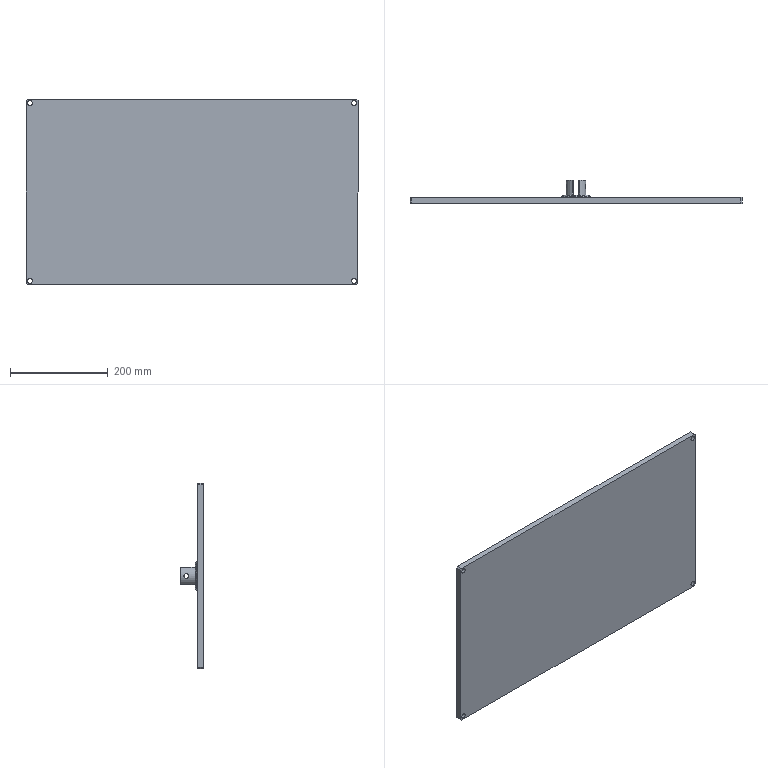Part | SolidWorks | features ICE 5, Chamfer 1, Extrusion 1 | 1 solid | 37 faces | box 680 x 47 x 380 mm | volume 3131077 mm3 | plane 19 | cylinder 16 | cone 2 | commonest cylinder face diameters 10 x12 40 x2 60 x2
STEP:
#1=CARTESIAN_POINT('',(-332.,0.,177.));
#2=VERTEX_POINT('',#1);
#3=CARTESIAN_POINT('',(-332.,0.,187.));
#4=VERTEX_POINT('',#3);
#5=CARTESIAN_POINT('',(-332.,0.,182.));
#6=DIRECTION('',(0.,1.,0.));
#7=DIRECTION('',(0.,0.,1.));
#8=AXIS2_PLACEMENT_3D('',#5,#6,#7);
#9=CIRCLE('',#8,5.);
#10=EDGE_CURVE('',#2,#4,#9,.T.);
#11=ORIENTED_EDGE('',*,*,#10,.F.);
#12=CARTESIAN_POINT('',(-332.,12.,177.));
#13=VERTEX_POINT('',#12);
#14=CARTESIAN_POINT('',(-332.,-18.,177.));
#15=DIRECTION('',(0.,1.,0.));
#16=VECTOR('',#15,1000.);
#17=LINE('',#14,#16);
#18=EDGE_CURVE('',#2,#13,#17,.T.);
#19=ORIENTED_EDGE('',*,*,#18,.T.);
#20=CARTESIAN_POINT('',(-332.,12.,187.));
#21=VERTEX_POINT('',#20);
#22=CARTESIAN_POINT('',(-332.,12.,182.));
#23=DIRECTION('',(0.,1.,0.));
#24=DIRECTION('',(0.,0.,-1.));
#25=AXIS2_PLACEMENT_3D('',#22,#23,#24);
#26=CIRCLE('',#25,5.);
#27=EDGE_CURVE('',#13,#21,#26,.T.);
#28=ORIENTED_EDGE('',*,*,#27,.T.);
#29=CARTESIAN_POINT('',(-332.,-18.,187.));
#30=DIRECTION('',(0.,1.,0.));
#31=VECTOR('',#30,1000.);
#32=LINE('',#29,#31);
#33=EDGE_CURVE('',#4,#21,#32,.T.);
#34=ORIENTED_EDGE('',*,*,#33,.F.);
#35=EDGE_LOOP('',(#11,#19,#28,#34));
#36=FACE_OUTER_BOUND('',#35,.T.);
#37=CARTESIAN_POINT('',(-332.,-18.,182.));
#38=DIRECTION('',(0.,1.,0.));
#39=DIRECTION('',(0.,0.,1.));
#40=AXIS2_PLACEMENT_3D('',#37,#38,#39);
#41=CYLINDRICAL_SURFACE('',#40,5.);
#42=ADVANCED_FACE('',(#36),#41,.F.);
#43=CARTESIAN_POINT('',(332.,0.,177.));
#44=VERTEX_POINT('',#43);
#45=CARTESIAN_POINT('',(332.,0.,187.));
#46=VERTEX_POINT('',#45);
#47=CARTESIAN_POINT('',(332.,0.,182.));
#48=DIRECTION('',(0.,1.,0.));
#49=DIRECTION('',(0.,0.,1.));
#50=AXIS2_PLACEMENT_3D('',#47,#48,#49);
#51=CIRCLE('',#50,5.);
#52=EDGE_CURVE('',#44,#46,#51,.T.);
#53=ORIENTED_EDGE('',*,*,#52,.F.);
#54=CARTESIAN_POINT('',(332.,12.,177.));
#55=VERTEX_POINT('',#54);
#56=CARTESIAN_POINT('',(332.,-18.,177.));
#57=DIRECTION('',(0.,1.,0.));
#58=VECTOR('',#57,1000.);
#59=LINE('',#56,#58);
#60=EDGE_CURVE('',#44,#55,#59,.T.);
#61=ORIENTED_EDGE('',*,*,#60,.T.);
#62=CARTESIAN_POINT('',(332.,12.,187.));
#63=VERTEX_POINT('',#62);
#64=CARTESIAN_POINT('',(332.,12.,182.));
#65=DIRECTION('',(0.,1.,0.));
#66=DIRECTION('',(0.,0.,1.));
#67=AXIS2_PLACEMENT_3D('',#64,#65,#66);
#68=CIRCLE('',#67,5.);
#69=EDGE_CURVE('',#55,#63,#68,.T.);
#70=ORIENTED_EDGE('',*,*,#69,.T.);
#71=CARTESIAN_POINT('',(332.,-18.,187.));
#72=DIRECTION('',(0.,1.,0.));
#73=VECTOR('',#72,1000.);
#74=LINE('',#71,#73);
#75=EDGE_CURVE('',#46,#63,#74,.T.);
#76=ORIENTED_EDGE('',*,*,#75,.F.);
#77=EDGE_LOOP('',(#53,#61,#70,#76));
#78=FACE_OUTER_BOUND('',#77,.T.);
#79=CARTESIAN_POINT('',(332.,-18.,182.));
#80=DIRECTION('',(0.,1.,0.));
#81=DIRECTION('',(0.,0.,1.));
#82=AXIS2_PLACEMENT_3D('',#79,#80,#81);
#83=CYLINDRICAL_SURFACE('',#82,5.);
#84=ADVANCED_FACE('',(#78),#83,.F.);
#85=CARTESIAN_POINT('',(332.,0.,-187.));
#86=VERTEX_POINT('',#85);
#87=CARTESIAN_POINT('',(332.,0.,-177.));
#88=VERTEX_POINT('',#87);
#89=CARTESIAN_POINT('',(332.,0.,-182.));
#90=DIRECTION('',(0.,1.,0.));
#91=DIRECTION('',(0.,0.,1.));
#92=AXIS2_PLACEMENT_3D('',#89,#90,#91);
#93=CIRCLE('',#92,5.);
#94=EDGE_CURVE('',#86,#88,#93,.T.);
#95=ORIENTED_EDGE('',*,*,#94,.F.);
#96=CARTESIAN_POINT('',(332.,12.,-187.));
#97=VERTEX_POINT('',#96);
#98=CARTESIAN_POINT('',(332.,-18.,-187.));
#99=DIRECTION('',(0.,1.,0.));
#100=VECTOR('',#99,1000.);
#101=LINE('',#98,#100);
#102=EDGE_CURVE('',#86,#97,#101,.T.);
#103=ORIENTED_EDGE('',*,*,#102,.T.);
#104=CARTESIAN_POINT('',(332.,12.,-177.));
#105=VERTEX_POINT('',#104);
#106=CARTESIAN_POINT('',(332.,12.,-182.));
#107=DIRECTION('',(0.,1.,0.));
#108=DIRECTION('',(0.,0.,-1.));
#109=AXIS2_PLACEMENT_3D('',#106,#107,#108);
#110=CIRCLE('',#109,5.);
#111=EDGE_CURVE('',#97,#105,#110,.T.);
#112=ORIENTED_EDGE('',*,*,#111,.T.);
#113=CARTESIAN_POINT('',(332.,-18.,-177.));
#114=DIRECTION('',(0.,1.,0.));
#115=VECTOR('',#114,1000.);
#116=LINE('',#113,#115);
#117=EDGE_CURVE('',#88,#105,#116,.T.);
#118=ORIENTED_EDGE('',*,*,#117,.F.);
#119=EDGE_LOOP('',(#95,#103,#112,#118));
#120=FACE_OUTER_BOUND('',#119,.T.);
#121=CARTESIAN_POINT('',(332.,-18.,-182.));
#122=DIRECTION('',(0.,1.,0.));
#123=DIRECTION('',(0.,0.,1.));
#124=AXIS2_PLACEMENT_3D('',#121,#122,#123);
#125=CYLINDRICAL_SURFACE('',#124,5.);
#126=ADVANCED_FACE('',(#120),#125,.F.);
#127=CARTESIAN_POINT('',(-332.,0.,-187.));
#128=VERTEX_POINT('',#127);
#129=CARTESIAN_POINT('',(-332.,0.,-177.));
#130=VERTEX_POINT('',#129);
#131=CARTESIAN_POINT('',(-332.,0.,-182.));
#132=DIRECTION('',(0.,1.,0.));
#133=DIRECTION('',(0.,0.,1.));
#134=AXIS2_PLACEMENT_3D('',#131,#132,#133);
#135=CIRCLE('',#134,5.);
#136=EDGE_CURVE('',#128,#130,#135,.T.);
#137=ORIENTED_EDGE('',*,*,#136,.F.);
#138=CARTESIAN_POINT('',(-332.,12.,-187.));
#139=VERTEX_POINT('',#138);
#140=CARTESIAN_POINT('',(-332.,-18.,-187.));
#141=DIRECTION('',(0.,1.,0.));
#142=VECTOR('',#141,1000.);
#143=LINE('',#140,#142);
#144=EDGE_CURVE('',#128,#139,#143,.T.);
#145=ORIENTED_EDGE('',*,*,#144,.T.);
#146=CARTESIAN_POINT('',(-332.,12.,-177.));
#147=VERTEX_POINT('',#146);
#148=CARTESIAN_POINT('',(-332.,12.,-182.));
#149=DIRECTION('',(0.,1.,0.));
#150=DIRECTION('',(0.,0.,1.));
#151=AXIS2_PLACEMENT_3D('',#148,#149,#150);
#152=CIRCLE('',#151,5.);
#153=EDGE_CURVE('',#139,#147,#152,.T.);
#154=ORIENTED_EDGE('',*,*,#153,.T.);
#155=CARTESIAN_POINT('',(-332.,-18.,-177.));
#156=DIRECTION('',(0.,1.,0.));
#157=VECTOR('',#156,1000.);
#158=LINE('',#155,#157);
#159=EDGE_CURVE('',#130,#147,#158,.T.);
#160=ORIENTED_EDGE('',*,*,#159,.F.);
#161=EDGE_LOOP('',(#137,#145,#154,#160));
#162=FACE_OUTER_BOUND('',#161,.T.);
#163=CARTESIAN_POINT('',(-332.,-18.,-182.));
#164=DIRECTION('',(0.,1.,0.));
#165=DIRECTION('',(0.,0.,1.));
#166=AXIS2_PLACEMENT_3D('',#163,#164,#165);
#167=CYLINDRICAL_SURFACE('',#166,5.);
#168=ADVANCED_FACE('',(#162),#167,.F.);
#169=CARTESIAN_POINT('',(0.,17.,27.));
#170=VERTEX_POINT('',#169);
#171=CARTESIAN_POINT('',(0.,17.,-27.));
#172=VERTEX_POINT('',#171);
#173=CARTESIAN_POINT('',(0.,17.,0.));
#174=DIRECTION('',(0.,1.,0.));
#175=DIRECTION('',(0.,0.,1.));
#176=AXIS2_PLACEMENT_3D('',#173,#174,#175);
#177=CIRCLE('',#176,27.);
#178=EDGE_CURVE('',#170,#172,#177,.T.);
#179=ORIENTED_EDGE('',*,*,#178,.F.);
#180=CARTESIAN_POINT('',(0.,14.,30.));
#181=VERTEX_POINT('',#180);
#182=CARTESIAN_POINT('',(0.,17.,27.));
#183=DIRECTION('',(0.,-0.7071,0.7071));
#184=VECTOR('',#183,1000.);
#185=LINE('',#182,#184);
#186=EDGE_CURVE('',#170,#181,#185,.T.);
#187=ORIENTED_EDGE('',*,*,#186,.T.);
#188=CARTESIAN_POINT('',(0.,14.,-30.));
#189=VERTEX_POINT('',#188);
#190=CARTESIAN_POINT('',(0.,14.,0.));
#191=DIRECTION('',(0.,-1.,0.));
#192=DIRECTION('',(0.,0.,1.));
#193=AXIS2_PLACEMENT_3D('',#190,#191,#192);
#194=CIRCLE('',#193,30.);
#195=EDGE_CURVE('',#189,#181,#194,.T.);
#196=ORIENTED_EDGE('',*,*,#195,.F.);
#197=CARTESIAN_POINT('',(0.,17.,-27.));
#198=DIRECTION('',(0.,-0.7071,-0.7071));
#199=VECTOR('',#198,1000.);
#200=LINE('',#197,#199);
#201=EDGE_CURVE('',#172,#189,#200,.T.);
#202=ORIENTED_EDGE('',*,*,#201,.F.);
#203=EDGE_LOOP('',(#179,#187,#196,#202));
#204=FACE_OUTER_BOUND('',#203,.T.);
#205=CARTESIAN_POINT('',(0.,17.,0.));
#206=DIRECTION('',(0.,-1.,0.));
#207=DIRECTION('',(0.,0.,-1.));
#208=AXIS2_PLACEMENT_3D('',#205,#206,#207);
#209=CONICAL_SURFACE('',#208,27.,0.7854);
#210=ADVANCED_FACE('',(#204),#209,.T.);
#211=CARTESIAN_POINT('',(-19.365,35.,5.));
#212=VERTEX_POINT('',#211);
#213=CARTESIAN_POINT('',(-19.365,35.,-5.));
#214=VERTEX_POINT('',#213);
#215=CARTESIAN_POINT('',(-19.365,35.,5.));
#216=CARTESIAN_POINT('',(-19.365,34.673,5.));
#217=CARTESIAN_POINT('',(-19.373,34.347,4.968));
#218=CARTESIAN_POINT('',(-19.406,33.697,4.839));
#219=CARTESIAN_POINT('',(-19.43,33.385,4.743));
#220=CARTESIAN_POINT('',(-19.489,32.782,4.493));
#221=CARTESIAN_POINT('',(-19.525,32.49,4.337));
#222=CARTESIAN_POINT('',(-19.602,31.948,3.974));
#223=CARTESIAN_POINT('',(-19.643,31.697,3.768));
#224=CARTESIAN_POINT('',(-19.726,31.236,3.307));
#225=CARTESIAN_POINT('',(-19.768,31.025,3.051));
#226=CARTESIAN_POINT('',(-19.844,30.664,2.511));
#227=CARTESIAN_POINT('',(-19.878,30.51,2.224));
#228=CARTESIAN_POINT('',(-19.937,30.257,1.616));
#229=CARTESIAN_POINT('',(-19.96,30.161,1.301));
#230=CARTESIAN_POINT('',(-19.984,30.065,0.8214));
#231=CARTESIAN_POINT('',(-19.99,30.041,0.6596));
#232=CARTESIAN_POINT('',(-19.998,30.008,0.3326));
#233=CARTESIAN_POINT('',(-20.,30.,0.1664));
#234=CARTESIAN_POINT('',(-20.,30.,-0.3283));
#235=CARTESIAN_POINT('',(-19.992,30.032,-0.6537));
#236=CARTESIAN_POINT('',(-19.961,30.16,-1.296));
#237=CARTESIAN_POINT('',(-19.937,30.257,-1.615));
#238=CARTESIAN_POINT('',(-19.879,30.507,-2.218));
#239=CARTESIAN_POINT('',(-19.844,30.661,-2.505));
#240=CARTESIAN_POINT('',(-19.768,31.025,-3.051));
#241=CARTESIAN_POINT('',(-19.727,31.233,-3.304));
#242=CARTESIAN_POINT('',(-19.644,31.692,-3.763));
#243=CARTESIAN_POINT('',(-19.602,31.946,-3.972));
#244=CARTESIAN_POINT('',(-19.525,32.49,-4.337));
#245=CARTESIAN_POINT('',(-19.49,32.777,-4.49));
#246=CARTESIAN_POINT('',(-19.43,33.379,-4.741));
#247=CARTESIAN_POINT('',(-19.406,33.697,-4.838));
#248=CARTESIAN_POINT('',(-19.373,34.341,-4.967));
#249=CARTESIAN_POINT('',(-19.365,34.668,-5.));
#250=CARTESIAN_POINT('',(-19.365,35.,-5.));
#251=B_SPLINE_CURVE_WITH_KNOTS('',3,(#215,#216,#217,#218,#219,#220,#221,#222,#223,#224,#225,#226,#227,#228,#229,#230,#231,#232,#233,#234,#235,#236,#237,#238,#239,#240,#241,#242,#243,#244,#245,#246,#247,#248,#249,#250),.UNSPECIFIED.,.F.,.F.,(4,2,2,2,2,2,2,2,2,2,2,2,2,2,2,2,2,4),(0.01569,0.01668,0.01766,0.01864,0.01962,0.0206,0.02158,0.02256,0.02305,0.02354,0.02452,0.0255,0.02648,0.02746,0.02844,0.02942,0.0304,0.03138),.UNSPECIFIED.);
#252=EDGE_CURVE('',#212,#214,#251,.T.);
#253=ORIENTED_EDGE('',*,*,#252,.F.);
#254=CARTESIAN_POINT('',(-6.,35.,5.));
#255=VERTEX_POINT('',#254);
#256=CARTESIAN_POINT('',(-340.,35.,5.));
#257=DIRECTION('',(1.,0.,0.));
#258=VECTOR('',#257,1000.);
#259=LINE('',#256,#258);
#260=EDGE_CURVE('',#212,#255,#259,.T.);
#261=ORIENTED_EDGE('',*,*,#260,.T.);
#262=CARTESIAN_POINT('',(-6.,35.,-5.));
#263=VERTEX_POINT('',#262);
#264=CARTESIAN_POINT('',(-6.,35.,0.));
#265=DIRECTION('',(1.,0.,0.));
#266=DIRECTION('',(0.,0.,1.));
#267=AXIS2_PLACEMENT_3D('',#264,#265,#266);
#268=CIRCLE('',#267,5.);
#269=EDGE_CURVE('',#255,#263,#268,.T.);
#270=ORIENTED_EDGE('',*,*,#269,.T.);
#271=CARTESIAN_POINT('',(-340.,35.,-5.));
#272=DIRECTION('',(1.,0.,0.));
#273=VECTOR('',#272,1000.);
#274=LINE('',#271,#273);
#275=EDGE_CURVE('',#214,#263,#274,.T.);
#276=ORIENTED_EDGE('',*,*,#275,.F.);
#277=EDGE_LOOP('',(#253,#261,#270,#276));
#278=FACE_OUTER_BOUND('',#277,.T.);
#279=CARTESIAN_POINT('',(-340.,35.,0.));
#280=DIRECTION('',(1.,0.,0.));
#281=DIRECTION('',(0.,0.,-1.));
#282=AXIS2_PLACEMENT_3D('',#279,#280,#281);
#283=CYLINDRICAL_SURFACE('',#282,5.);
#284=ADVANCED_FACE('',(#278),#283,.F.);
#285=CARTESIAN_POINT('',(6.,35.,-5.));
#286=VERTEX_POINT('',#285);
#287=CARTESIAN_POINT('',(6.,35.,5.));
#288=VERTEX_POINT('',#287);
#289=CARTESIAN_POINT('',(6.,35.,0.));
#290=DIRECTION('',(-1.,0.,0.));
#291=DIRECTION('',(0.,0.,-1.));
#292=AXIS2_PLACEMENT_3D('',#289,#290,#291);
#293=CIRCLE('',#292,5.);
#294=EDGE_CURVE('',#286,#288,#293,.T.);
#295=ORIENTED_EDGE('',*,*,#294,.T.);
#296=CARTESIAN_POINT('',(19.365,35.,5.));
#297=VERTEX_POINT('',#296);
#298=CARTESIAN_POINT('',(-340.,35.,5.));
#299=DIRECTION('',(1.,0.,0.));
#300=VECTOR('',#299,1000.);
#301=LINE('',#298,#300);
#302=EDGE_CURVE('',#288,#297,#301,.T.);
#303=ORIENTED_EDGE('',*,*,#302,.T.);
#304=CARTESIAN_POINT('',(19.365,35.,-5.));
#305=VERTEX_POINT('',#304);
#306=CARTESIAN_POINT('',(19.365,35.,-5.));
#307=CARTESIAN_POINT('',(19.365,34.668,-5.));
#308=CARTESIAN_POINT('',(19.373,34.342,-4.967));
#309=CARTESIAN_POINT('',(19.406,33.701,-4.839));
#310=CARTESIAN_POINT('',(19.43,33.383,-4.743));
#311=CARTESIAN_POINT('',(19.49,32.778,-4.491));
#312=CARTESIAN_POINT('',(19.525,32.492,-4.338));
#313=CARTESIAN_POINT('',(19.602,31.949,-3.975));
#314=CARTESIAN_POINT('',(19.644,31.693,-3.764));
#315=CARTESIAN_POINT('',(19.726,31.234,-3.305));
#316=CARTESIAN_POINT('',(19.767,31.028,-3.054));
#317=CARTESIAN_POINT('',(19.844,30.662,-2.508));
#318=CARTESIAN_POINT('',(19.879,30.508,-2.219));
#319=CARTESIAN_POINT('',(19.922,30.32,-1.768));
#320=CARTESIAN_POINT('',(19.935,30.265,-1.614));
#321=CARTESIAN_POINT('',(19.958,30.169,-1.301));
#322=CARTESIAN_POINT('',(19.968,30.129,-1.14));
#323=CARTESIAN_POINT('',(19.992,30.032,-0.655));
#324=CARTESIAN_POINT('',(20.,30.,-0.3296));
#325=CARTESIAN_POINT('',(20.,30.,0.3256));
#326=CARTESIAN_POINT('',(19.992,30.033,0.6584));
#327=CARTESIAN_POINT('',(19.96,30.161,1.301));
#328=CARTESIAN_POINT('',(19.937,30.256,1.613));
#329=CARTESIAN_POINT('',(19.879,30.508,2.22));
#330=CARTESIAN_POINT('',(19.844,30.664,2.511));
#331=CARTESIAN_POINT('',(19.768,31.025,3.051));
#332=CARTESIAN_POINT('',(19.726,31.234,3.305));
#333=CARTESIAN_POINT('',(19.643,31.697,3.768));
#334=CARTESIAN_POINT('',(19.602,31.948,3.974));
#335=CARTESIAN_POINT('',(19.525,32.489,4.336));
#336=CARTESIAN_POINT('',(19.489,32.782,4.493));
#337=CARTESIAN_POINT('',(19.43,33.385,4.743));
#338=CARTESIAN_POINT('',(19.406,33.697,4.838));
#339=CARTESIAN_POINT('',(19.382,34.18,4.935));
#340=CARTESIAN_POINT('',(19.375,34.344,4.96));
#341=CARTESIAN_POINT('',(19.367,34.673,4.992));
#342=CARTESIAN_POINT('',(19.365,34.836,5.));
#343=CARTESIAN_POINT('',(19.365,35.,5.));
#344=B_SPLINE_CURVE_WITH_KNOTS('',3,(#306,#307,#308,#309,#310,#311,#312,#313,#314,#315,#316,#317,#318,#319,#320,#321,#322,#323,#324,#325,#326,#327,#328,#329,#330,#331,#332,#333,#334,#335,#336,#337,#338,#339,#340,#341,#342,#343),.UNSPECIFIED.,.F.,.F.,(4,2,2,2,2,2,2,2,2,2,2,2,2,2,2,2,2,2,4),(0.,0.0009809,0.001962,0.002943,0.003924,0.004905,0.005885,0.006376,0.006866,0.007847,0.008828,0.009809,0.01079,0.01177,0.01275,0.01373,0.01471,0.0152,0.01569),.UNSPECIFIED.);
#345=EDGE_CURVE('',#305,#297,#344,.T.);
#346=ORIENTED_EDGE('',*,*,#345,.F.);
#347=CARTESIAN_POINT('',(-340.,35.,-5.));
#348=DIRECTION('',(1.,0.,0.));
#349=VECTOR('',#348,1000.);
#350=LINE('',#347,#349);
#351=EDGE_CURVE('',#286,#305,#350,.T.);
#352=ORIENTED_EDGE('',*,*,#351,.F.);
#353=EDGE_LOOP('',(#295,#303,#346,#352));
#354=FACE_OUTER_BOUND('',#353,.T.);
#355=CARTESIAN_POINT('',(-340.,35.,0.));
#356=DIRECTION('',(1.,0.,0.));
#357=DIRECTION('',(0.,0.,-1.));
#358=AXIS2_PLACEMENT_3D('',#355,#356,#357);
#359=CYLINDRICAL_SURFACE('',#358,5.);
#360=ADVANCED_FACE('',(#354),#359,.F.);
#361=ORIENTED_EDGE('',*,*,#195,.T.);
#362=CARTESIAN_POINT('',(0.,12.,30.));
#363=VERTEX_POINT('',#362);
#364=CARTESIAN_POINT('',(0.,17.,30.));
#365=DIRECTION('',(0.,-1.,0.));
#366=VECTOR('',#365,1000.);
#367=LINE('',#364,#366);
#368=EDGE_CURVE('',#181,#363,#367,.T.);
#369=ORIENTED_EDGE('',*,*,#368,.T.);
#370=CARTESIAN_POINT('',(0.,12.,-30.));
#371=VERTEX_POINT('',#370);
#372=CARTESIAN_POINT('',(0.,12.,0.));
#373=DIRECTION('',(0.,1.,0.));
#374=DIRECTION('',(0.,0.,1.));
#375=AXIS2_PLACEMENT_3D('',#372,#373,#374);
#376=CIRCLE('',#375,30.);
#377=EDGE_CURVE('',#363,#371,#376,.T.);
#378=ORIENTED_EDGE('',*,*,#377,.T.);
#379=CARTESIAN_POINT('',(0.,17.,-30.));
#380=DIRECTION('',(0.,-1.,0.));
#381=VECTOR('',#380,1000.);
#382=LINE('',#379,#381);
#383=EDGE_CURVE('',#189,#371,#382,.T.);
#384=ORIENTED_EDGE('',*,*,#383,.F.);
#385=EDGE_LOOP('',(#361,#369,#378,#384));
#386=FACE_OUTER_BOUND('',#385,.T.);
#387=CARTESIAN_POINT('',(0.,17.,0.));
#388=DIRECTION('',(0.,-1.,0.));
#389=DIRECTION('',(0.,0.,-1.));
#390=AXIS2_PLACEMENT_3D('',#387,#388,#389);
#391=CYLINDRICAL_SURFACE('',#390,30.);
#392=ADVANCED_FACE('',(#386),#391,.T.);
#393=CARTESIAN_POINT('',(340.,0.,187.));
#394=VERTEX_POINT('',#393);
#395=CARTESIAN_POINT('',(340.,0.,-187.));
#396=VERTEX_POINT('',#395);
#397=CARTESIAN_POINT('',(340.,0.,-190.));
#398=DIRECTION('',(0.,0.,-1.));
#399=VECTOR('',#398,1000.);
#400=LINE('',#397,#399);
#401=EDGE_CURVE('',#394,#396,#400,.T.);
#402=ORIENTED_EDGE('',*,*,#401,.T.);
#403=CARTESIAN_POINT('',(340.,12.,-187.));
#404=VERTEX_POINT('',#403);
#405=CARTESIAN_POINT('',(340.,12.,-187.));
#406=DIRECTION('',(0.,1.,0.));
#407=VECTOR('',#406,1000.);
#408=LINE('',#405,#407);
#409=EDGE_CURVE('',#396,#404,#408,.T.);
#410=ORIENTED_EDGE('',*,*,#409,.T.);
#411=CARTESIAN_POINT('',(340.,12.,187.));
#412=VERTEX_POINT('',#411);
#413=CARTESIAN_POINT('',(340.,12.,-190.));
#414=DIRECTION('',(0.,0.,-1.));
#415=VECTOR('',#414,1000.);
#416=LINE('',#413,#415);
#417=EDGE_CURVE('',#412,#404,#416,.T.);
#418=ORIENTED_EDGE('',*,*,#417,.F.);
#419=CARTESIAN_POINT('',(340.,12.,187.));
#420=DIRECTION('',(0.,-1.,0.));
#421=VECTOR('',#420,1000.);
#422=LINE('',#419,#421);
#423=EDGE_CURVE('',#412,#394,#422,.T.);
#424=ORIENTED_EDGE('',*,*,#423,.T.);
#425=EDGE_LOOP('',(#402,#410,#418,#424));
#426=FACE_OUTER_BOUND('',#425,.T.);
#427=CARTESIAN_POINT('',(340.,12.,-190.));
#428=DIRECTION('',(-1.,0.,0.));
#429=DIRECTION('',(0.,0.,1.));
#430=AXIS2_PLACEMENT_3D('',#427,#428,#429);
#431=PLANE('',#430);
#432=ADVANCED_FACE('',(#426),#431,.F.);
#433=CARTESIAN_POINT('',(337.,0.,-190.));
#434=VERTEX_POINT('',#433);
#435=CARTESIAN_POINT('',(-337.,0.,-190.));
#436=VERTEX_POINT('',#435);
#437=CARTESIAN_POINT('',(-340.,0.,-190.));
#438=DIRECTION('',(-1.,0.,0.));
#439=VECTOR('',#438,1000.);
#440=LINE('',#437,#439);
#441=EDGE_CURVE('',#434,#436,#440,.T.);
#442=ORIENTED_EDGE('',*,*,#441,.T.);
#443=CARTESIAN_POINT('',(-337.,12.,-190.));
#444=VERTEX_POINT('',#443);
#445=CARTESIAN_POINT('',(-337.,12.,-190.));
#446=DIRECTION('',(0.,1.,0.));
#447=VECTOR('',#446,1000.);
#448=LINE('',#445,#447);
#449=EDGE_CURVE('',#436,#444,#448,.T.);
#450=ORIENTED_EDGE('',*,*,#449,.T.);
#451=CARTESIAN_POINT('',(337.,12.,-190.));
#452=VERTEX_POINT('',#451);
#453=CARTESIAN_POINT('',(-340.,12.,-190.));
#454=DIRECTION('',(-1.,0.,0.));
#455=VECTOR('',#454,1000.);
#456=LINE('',#453,#455);
#457=EDGE_CURVE('',#452,#444,#456,.T.);
#458=ORIENTED_EDGE('',*,*,#457,.F.);
#459=CARTESIAN_POINT('',(337.,12.,-190.));
#460=DIRECTION('',(0.,-1.,0.));
#461=VECTOR('',#460,1000.);
#462=LINE('',#459,#461);
#463=EDGE_CURVE('',#452,#434,#462,.T.);
#464=ORIENTED_EDGE('',*,*,#463,.T.);
#465=EDGE_LOOP('',(#442,#450,#458,#464));
#466=FACE_OUTER_BOUND('',#465,.T.);
#467=CARTESIAN_POINT('',(-340.,12.,-190.));
#468=DIRECTION('',(0.,0.,1.));
#469=DIRECTION('',(1.,0.,0.));
#470=AXIS2_PLACEMENT_3D('',#467,#468,#469);
#471=PLANE('',#470);
#472=ADVANCED_FACE('',(#466),#471,.F.);
#473=CARTESIAN_POINT('',(-340.,12.,-187.));
#474=VERTEX_POINT('',#473);
#475=CARTESIAN_POINT('',(-340.,12.,187.));
#476=VERTEX_POINT('',#475);
#477=CARTESIAN_POINT('',(-340.,12.,-190.));
#478=DIRECTION('',(0.,0.,1.));
#479=VECTOR('',#478,1000.);
#480=LINE('',#477,#479);
#481=EDGE_CURVE('',#474,#476,#480,.T.);
#482=ORIENTED_EDGE('',*,*,#481,.F.);
#483=CARTESIAN_POINT('',(-340.,0.,-187.));
#484=VERTEX_POINT('',#483);
#485=CARTESIAN_POINT('',(-340.,12.,-187.));
#486=DIRECTION('',(0.,-1.,0.));
#487=VECTOR('',#486,1000.);
#488=LINE('',#485,#487);
#489=EDGE_CURVE('',#474,#484,#488,.T.);
#490=ORIENTED_EDGE('',*,*,#489,.T.);
#491=CARTESIAN_POINT('',(-340.,0.,187.));
#492=VERTEX_POINT('',#491);
#493=CARTESIAN_POINT('',(-340.,0.,-190.));
#494=DIRECTION('',(0.,0.,1.));
#495=VECTOR('',#494,1000.);
#496=LINE('',#493,#495);
#497=EDGE_CURVE('',#484,#492,#496,.T.);
#498=ORIENTED_EDGE('',*,*,#497,.T.);
#499=CARTESIAN_POINT('',(-340.,12.,187.));
#500=DIRECTION('',(0.,1.,0.));
#501=VECTOR('',#500,1000.);
#502=LINE('',#499,#501);
#503=EDGE_CURVE('',#492,#476,#502,.T.);
#504=ORIENTED_EDGE('',*,*,#503,.T.);
#505=EDGE_LOOP('',(#482,#490,#498,#504));
#506=FACE_OUTER_BOUND('',#505,.T.);
#507=CARTESIAN_POINT('',(-340.,12.,-190.));
#508=DIRECTION('',(1.,0.,0.));
#509=DIRECTION('',(0.,0.,-1.));
#510=AXIS2_PLACEMENT_3D('',#507,#508,#509);
#511=PLANE('',#510);
#512=ADVANCED_FACE('',(#506),#511,.F.);
#513=CARTESIAN_POINT('',(-337.,0.,190.));
#514=VERTEX_POINT('',#513);
#515=CARTESIAN_POINT('',(337.,0.,190.));
#516=VERTEX_POINT('',#515);
#517=CARTESIAN_POINT('',(-340.,0.,190.));
#518=DIRECTION('',(1.,0.,0.));
#519=VECTOR('',#518,1000.);
#520=LINE('',#517,#519);
#521=EDGE_CURVE('',#514,#516,#520,.T.);
#522=ORIENTED_EDGE('',*,*,#521,.T.);
#523=CARTESIAN_POINT('',(337.,12.,190.));
#524=VERTEX_POINT('',#523);
#525=CARTESIAN_POINT('',(337.,12.,190.));
#526=DIRECTION('',(0.,1.,0.));
#527=VECTOR('',#526,1000.);
#528=LINE('',#525,#527);
#529=EDGE_CURVE('',#516,#524,#528,.T.);
#530=ORIENTED_EDGE('',*,*,#529,.T.);
#531=CARTESIAN_POINT('',(-337.,12.,190.));
#532=VERTEX_POINT('',#531);
#533=CARTESIAN_POINT('',(-340.,12.,190.));
#534=DIRECTION('',(1.,0.,0.));
#535=VECTOR('',#534,1000.);
#536=LINE('',#533,#535);
#537=EDGE_CURVE('',#532,#524,#536,.T.);
#538=ORIENTED_EDGE('',*,*,#537,.F.);
#539=CARTESIAN_POINT('',(-337.,12.,190.));
#540=DIRECTION('',(0.,-1.,0.));
#541=VECTOR('',#540,1000.);
#542=LINE('',#539,#541);
#543=EDGE_CURVE('',#532,#514,#542,.T.);
#544=ORIENTED_EDGE('',*,*,#543,.T.);
#545=EDGE_LOOP('',(#522,#530,#538,#544));
#546=FACE_OUTER_BOUND('',#545,.T.);
#547=CARTESIAN_POINT('',(-340.,12.,190.));
#548=DIRECTION('',(0.,0.,-1.));
#549=DIRECTION('',(-1.,0.,0.));
#550=AXIS2_PLACEMENT_3D('',#547,#548,#549);
#551=PLANE('',#550);
#552=ADVANCED_FACE('',(#546),#551,.F.);
#553=CARTESIAN_POINT('',(-332.,12.,182.));
#554=DIRECTION('',(0.,1.,0.));
#555=DIRECTION('',(0.,0.,-1.));
#556=AXIS2_PLACEMENT_3D('',#553,#554,#555);
#557=CIRCLE('',#556,5.);
#558=EDGE_CURVE('',#21,#13,#557,.T.);
#559=ORIENTED_EDGE('',*,*,#558,.F.);
#560=ORIENTED_EDGE('',*,*,#27,.F.);
#561=EDGE_LOOP('',(#559,#560));
#562=FACE_BOUND('',#561,.T.);
#563=CARTESIAN_POINT('',(332.,12.,182.));
#564=DIRECTION('',(0.,1.,0.));
#565=DIRECTION('',(0.,0.,1.));
#566=AXIS2_PLACEMENT_3D('',#563,#564,#565);
#567=CIRCLE('',#566,5.);
#568=EDGE_CURVE('',#63,#55,#567,.T.);
#569=ORIENTED_EDGE('',*,*,#568,.F.);
#570=ORIENTED_EDGE('',*,*,#69,.F.);
#571=EDGE_LOOP('',(#569,#570));
#572=FACE_BOUND('',#571,.T.);
#573=CARTESIAN_POINT('',(332.,12.,-182.));
#574=DIRECTION('',(0.,1.,0.));
#575=DIRECTION('',(0.,0.,-1.));
#576=AXIS2_PLACEMENT_3D('',#573,#574,#575);
#577=CIRCLE('',#576,5.);
#578=EDGE_CURVE('',#105,#97,#577,.T.);
#579=ORIENTED_EDGE('',*,*,#578,.F.);
#580=ORIENTED_EDGE('',*,*,#111,.F.);
#581=EDGE_LOOP('',(#579,#580));
#582=FACE_BOUND('',#581,.T.);
#583=CARTESIAN_POINT('',(-332.,12.,-182.));
#584=DIRECTION('',(0.,1.,0.));
#585=DIRECTION('',(0.,0.,1.));
#586=AXIS2_PLACEMENT_3D('',#583,#584,#585);
#587=CIRCLE('',#586,5.);
#588=EDGE_CURVE('',#147,#139,#587,.T.);
#589=ORIENTED_EDGE('',*,*,#588,.F.);
#590=ORIENTED_EDGE('',*,*,#153,.F.);
#591=EDGE_LOOP('',(#589,#590));
#592=FACE_BOUND('',#591,.T.);
#593=CARTESIAN_POINT('',(0.,12.,0.));
#594=DIRECTION('',(0.,1.,0.));
#595=DIRECTION('',(0.,0.,1.));
#596=AXIS2_PLACEMENT_3D('',#593,#594,#595);
#597=CIRCLE('',#596,30.);
#598=EDGE_CURVE('',#371,#363,#597,.T.);
#599=ORIENTED_EDGE('',*,*,#598,.F.);
#600=ORIENTED_EDGE('',*,*,#377,.F.);
#601=EDGE_LOOP('',(#599,#600));
#602=FACE_BOUND('',#601,.T.);
#603=ORIENTED_EDGE('',*,*,#457,.T.);
#604=CARTESIAN_POINT('',(-263.5,12.,-263.5));
#605=DIRECTION('',(-0.7071,0.,0.7071));
#606=VECTOR('',#605,1000.);
#607=LINE('',#604,#606);
#608=EDGE_CURVE('',#444,#474,#607,.T.);
#609=ORIENTED_EDGE('',*,*,#608,.T.);
#610=ORIENTED_EDGE('',*,*,#481,.T.);
#611=CARTESIAN_POINT('',(-263.5,12.,263.5));
#612=DIRECTION('',(0.7071,0.,0.7071));
#613=VECTOR('',#612,1000.);
#614=LINE('',#611,#613);
#615=EDGE_CURVE('',#476,#532,#614,.T.);
#616=ORIENTED_EDGE('',*,*,#615,.T.);
#617=ORIENTED_EDGE('',*,*,#537,.T.);
#618=CARTESIAN_POINT('',(263.5,12.,263.5));
#619=DIRECTION('',(0.7071,0.,-0.7071));
#620=VECTOR('',#619,1000.);
#621=LINE('',#618,#620);
#622=EDGE_CURVE('',#524,#412,#621,.T.);
#623=ORIENTED_EDGE('',*,*,#622,.T.);
#624=ORIENTED_EDGE('',*,*,#417,.T.);
#625=CARTESIAN_POINT('',(263.5,12.,-263.5));
#626=DIRECTION('',(-0.7071,0.,-0.7071));
#627=VECTOR('',#626,1000.);
#628=LINE('',#625,#627);
#629=EDGE_CURVE('',#404,#452,#628,.T.);
#630=ORIENTED_EDGE('',*,*,#629,.T.);
#631=EDGE_LOOP('',(#603,#609,#610,#616,#617,#623,#624,#630));
#632=FACE_OUTER_BOUND('',#631,.T.);
#633=CARTESIAN_POINT('',(0.,12.,0.));
#634=DIRECTION('',(0.,1.,0.));
#635=DIRECTION('',(0.,0.,1.));
#636=AXIS2_PLACEMENT_3D('',#633,#634,#635);
#637=PLANE('',#636);
#638=ADVANCED_FACE('',(#562,#572,#582,#592,#602,#632),#637,.T.);
#639=CARTESIAN_POINT('',(-332.,0.,182.));
#640=DIRECTION('',(0.,1.,0.));
#641=DIRECTION('',(0.,0.,1.));
#642=AXIS2_PLACEMENT_3D('',#639,#640,#641);
#643=CIRCLE('',#642,5.);
#644=EDGE_CURVE('',#4,#2,#643,.T.);
#645=ORIENTED_EDGE('',*,*,#644,.T.);
#646=ORIENTED_EDGE('',*,*,#10,.T.);
#647=EDGE_LOOP('',(#645,#646));
#648=FACE_BOUND('',#647,.T.);
#649=CARTESIAN_POINT('',(332.,0.,182.));
#650=DIRECTION('',(0.,1.,0.));
#651=DIRECTION('',(0.,0.,1.));
#652=AXIS2_PLACEMENT_3D('',#649,#650,#651);
#653=CIRCLE('',#652,5.);
#654=EDGE_CURVE('',#46,#44,#653,.T.);
#655=ORIENTED_EDGE('',*,*,#654,.T.);
#656=ORIENTED_EDGE('',*,*,#52,.T.);
#657=EDGE_LOOP('',(#655,#656));
#658=FACE_BOUND('',#657,.T.);
#659=CARTESIAN_POINT('',(332.,0.,-182.));
#660=DIRECTION('',(0.,1.,0.));
#661=DIRECTION('',(0.,0.,1.));
#662=AXIS2_PLACEMENT_3D('',#659,#660,#661);
#663=CIRCLE('',#662,5.);
#664=EDGE_CURVE('',#88,#86,#663,.T.);
#665=ORIENTED_EDGE('',*,*,#664,.T.);
#666=ORIENTED_EDGE('',*,*,#94,.T.);
#667=EDGE_LOOP('',(#665,#666));
#668=FACE_BOUND('',#667,.T.);
#669=CARTESIAN_POINT('',(-332.,0.,-182.));
#670=DIRECTION('',(0.,1.,0.));
#671=DIRECTION('',(0.,0.,1.));
#672=AXIS2_PLACEMENT_3D('',#669,#670,#671);
#673=CIRCLE('',#672,5.);
#674=EDGE_CURVE('',#130,#128,#673,.T.);
#675=ORIENTED_EDGE('',*,*,#674,.T.);
#676=ORIENTED_EDGE('',*,*,#136,.T.);
#677=EDGE_LOOP('',(#675,#676));
#678=FACE_BOUND('',#677,.T.);
#679=ORIENTED_EDGE('',*,*,#497,.F.);
#680=CARTESIAN_POINT('',(-340.,0.,-187.));
#681=DIRECTION('',(0.7071,0.,-0.7071));
#682=VECTOR('',#681,1000.);
#683=LINE('',#680,#682);
#684=EDGE_CURVE('',#484,#436,#683,.T.);
#685=ORIENTED_EDGE('',*,*,#684,.T.);
#686=ORIENTED_EDGE('',*,*,#441,.F.);
#687=CARTESIAN_POINT('',(337.,0.,-190.));
#688=DIRECTION('',(0.7071,0.,0.7071));
#689=VECTOR('',#688,1000.);
#690=LINE('',#687,#689);
#691=EDGE_CURVE('',#434,#396,#690,.T.);
#692=ORIENTED_EDGE('',*,*,#691,.T.);
#693=ORIENTED_EDGE('',*,*,#401,.F.);
#694=CARTESIAN_POINT('',(340.,0.,187.));
#695=DIRECTION('',(-0.7071,0.,0.7071));
#696=VECTOR('',#695,1000.);
#697=LINE('',#694,#696);
#698=EDGE_CURVE('',#394,#516,#697,.T.);
#699=ORIENTED_EDGE('',*,*,#698,.T.);
#700=ORIENTED_EDGE('',*,*,#521,.F.);
#701=CARTESIAN_POINT('',(-337.,0.,190.));
#702=DIRECTION('',(-0.7071,0.,-0.7071));
#703=VECTOR('',#702,1000.);
#704=LINE('',#701,#703);
#705=EDGE_CURVE('',#514,#492,#704,.T.);
#706=ORIENTED_EDGE('',*,*,#705,.T.);
#707=EDGE_LOOP('',(#679,#685,#686,#692,#693,#699,#700,#706));
#708=FACE_OUTER_BOUND('',#707,.T.);
#709=CARTESIAN_POINT('',(0.,0.,0.));
#710=DIRECTION('',(0.,1.,0.));
#711=DIRECTION('',(0.,0.,1.));
#712=AXIS2_PLACEMENT_3D('',#709,#710,#711);
#713=PLANE('',#712);
#714=ADVANCED_FACE('',(#648,#658,#668,#678,#708),#713,.F.);
#715=CARTESIAN_POINT('',(0.,17.,0.));
#716=DIRECTION('',(0.,1.,0.));
#717=DIRECTION('',(0.,0.,1.));
#718=AXIS2_PLACEMENT_3D('',#715,#716,#717);
#719=CIRCLE('',#718,27.);
#720=EDGE_CURVE('',#172,#170,#719,.T.);
#721=ORIENTED_EDGE('',*,*,#720,.T.);
#722=ORIENTED_EDGE('',*,*,#178,.T.);
#723=EDGE_LOOP('',(#721,#722));
#724=FACE_OUTER_BOUND('',#723,.T.);
#725=CARTESIAN_POINT('',(-8.174,17.,-18.253));
#726=VERTEX_POINT('',#725);
#727=CARTESIAN_POINT('',(-8.174,17.,18.253));
#728=VERTEX_POINT('',#727);
#729=CARTESIAN_POINT('',(0.,17.,0.));
#730=DIRECTION('',(0.,1.,0.));
#731=DIRECTION('',(0.,0.,1.));
#732=AXIS2_PLACEMENT_3D('',#729,#730,#731);
#733=CIRCLE('',#732,20.);
#734=EDGE_CURVE('',#726,#728,#733,.T.);
#735=ORIENTED_EDGE('',*,*,#734,.F.);
#736=CARTESIAN_POINT('',(-6.,17.,-16.079));
#737=VERTEX_POINT('',#736);
#738=CARTESIAN_POINT('',(-8.174,17.,-18.253));
#739=DIRECTION('',(0.7071,0.,0.7071));
#740=VECTOR('',#739,1000.);
#741=LINE('',#738,#740);
#742=EDGE_CURVE('',#726,#737,#741,.T.);
#743=ORIENTED_EDGE('',*,*,#742,.T.);
#744=CARTESIAN_POINT('',(-6.,17.,16.079));
#745=VERTEX_POINT('',#744);
#746=CARTESIAN_POINT('',(-6.,17.,-46.332));
#747=DIRECTION('',(0.,0.,-1.));
#748=VECTOR('',#747,1000.);
#749=LINE('',#746,#748);
#750=EDGE_CURVE('',#745,#737,#749,.T.);
#751=ORIENTED_EDGE('',*,*,#750,.F.);
#752=CARTESIAN_POINT('',(-8.174,17.,18.253));
#753=DIRECTION('',(-0.7071,0.,0.7071));
#754=VECTOR('',#753,1000.);
#755=LINE('',#752,#754);
#756=EDGE_CURVE('',#745,#728,#755,.T.);
#757=ORIENTED_EDGE('',*,*,#756,.T.);
#758=EDGE_LOOP('',(#735,#743,#751,#757));
#759=FACE_BOUND('',#758,.T.);
#760=CARTESIAN_POINT('',(8.174,17.,18.253));
#761=VERTEX_POINT('',#760);
#762=CARTESIAN_POINT('',(8.174,17.,-18.253));
#763=VERTEX_POINT('',#762);
#764=CARTESIAN_POINT('',(0.,17.,0.));
#765=DIRECTION('',(0.,1.,0.));
#766=DIRECTION('',(0.,0.,1.));
#767=AXIS2_PLACEMENT_3D('',#764,#765,#766);
#768=CIRCLE('',#767,20.);
#769=EDGE_CURVE('',#761,#763,#768,.T.);
#770=ORIENTED_EDGE('',*,*,#769,.F.);
#771=CARTESIAN_POINT('',(6.,17.,16.079));
#772=VERTEX_POINT('',#771);
#773=CARTESIAN_POINT('',(8.174,17.,18.253));
#774=DIRECTION('',(-0.7071,0.,-0.7071));
#775=VECTOR('',#774,1000.);
#776=LINE('',#773,#775);
#777=EDGE_CURVE('',#761,#772,#776,.T.);
#778=ORIENTED_EDGE('',*,*,#777,.T.);
#779=CARTESIAN_POINT('',(6.,17.,-16.079));
#780=VERTEX_POINT('',#779);
#781=CARTESIAN_POINT('',(6.,17.,-46.332));
#782=DIRECTION('',(0.,0.,1.));
#783=VECTOR('',#782,1000.);
#784=LINE('',#781,#783);
#785=EDGE_CURVE('',#780,#772,#784,.T.);
#786=ORIENTED_EDGE('',*,*,#785,.F.);
#787=CARTESIAN_POINT('',(8.174,17.,-18.253));
#788=DIRECTION('',(0.7071,0.,-0.7071));
#789=VECTOR('',#788,1000.);
#790=LINE('',#787,#789);
#791=EDGE_CURVE('',#780,#763,#790,.T.);
#792=ORIENTED_EDGE('',*,*,#791,.T.);
#793=EDGE_LOOP('',(#770,#778,#786,#792));
#794=FACE_BOUND('',#793,.T.);
#795=CARTESIAN_POINT('',(0.,17.,0.));
#796=DIRECTION('',(0.,1.,0.));
#797=DIRECTION('',(0.,0.,1.));
#798=AXIS2_PLACEMENT_3D('',#795,#796,#797);
#799=PLANE('',#798);
#800=ADVANCED_FACE('',(#724,#759,#794),#799,.T.);
#801=ORIENTED_EDGE('',*,*,#368,.F.);
#802=CARTESIAN_POINT('',(0.,14.,0.));
#803=DIRECTION('',(0.,-1.,0.));
#804=DIRECTION('',(0.,0.,1.));
#805=AXIS2_PLACEMENT_3D('',#802,#803,#804);
#806=CIRCLE('',#805,30.);
#807=EDGE_CURVE('',#181,#189,#806,.T.);
#808=ORIENTED_EDGE('',*,*,#807,.T.);
#809=ORIENTED_EDGE('',*,*,#383,.T.);
#810=ORIENTED_EDGE('',*,*,#598,.T.);
#811=EDGE_LOOP('',(#801,#808,#809,#810));
#812=FACE_OUTER_BOUND('',#811,.T.);
#813=CARTESIAN_POINT('',(0.,17.,0.));
#814=DIRECTION('',(0.,-1.,0.));
#815=DIRECTION('',(0.,0.,-1.));
#816=AXIS2_PLACEMENT_3D('',#813,#814,#815);
#817=CYLINDRICAL_SURFACE('',#816,30.);
#818=ADVANCED_FACE('',(#812),#817,.T.);
#819=CARTESIAN_POINT('',(8.174,47.,18.253));
#820=VERTEX_POINT('',#819);
#821=CARTESIAN_POINT('',(8.174,47.,-18.253));
#822=VERTEX_POINT('',#821);
#823=CARTESIAN_POINT('',(0.,47.,0.));
#824=DIRECTION('',(0.,1.,0.));
#825=DIRECTION('',(0.,0.,1.));
#826=AXIS2_PLACEMENT_3D('',#823,#824,#825);
#827=CIRCLE('',#826,20.);
#828=EDGE_CURVE('',#820,#822,#827,.T.);
#829=ORIENTED_EDGE('',*,*,#828,.T.);
#830=CARTESIAN_POINT('',(6.,47.,-16.079));
#831=VERTEX_POINT('',#830);
#832=CARTESIAN_POINT('',(-5.039,47.,-5.039));
#833=DIRECTION('',(-0.7071,0.,0.7071));
#834=VECTOR('',#833,1000.);
#835=LINE('',#832,#834);
#836=EDGE_CURVE('',#822,#831,#835,.T.);
#837=ORIENTED_EDGE('',*,*,#836,.T.);
#838=CARTESIAN_POINT('',(6.,47.,16.079));
#839=VERTEX_POINT('',#838);
#840=CARTESIAN_POINT('',(6.,47.,-46.332));
#841=DIRECTION('',(0.,0.,-1.));
#842=VECTOR('',#841,1000.);
#843=LINE('',#840,#842);
#844=EDGE_CURVE('',#839,#831,#843,.T.);
#845=ORIENTED_EDGE('',*,*,#844,.F.);
#846=CARTESIAN_POINT('',(-5.039,47.,5.039));
#847=DIRECTION('',(0.7071,0.,0.7071));
#848=VECTOR('',#847,1000.);
#849=LINE('',#846,#848);
#850=EDGE_CURVE('',#839,#820,#849,.T.);
#851=ORIENTED_EDGE('',*,*,#850,.T.);
#852=EDGE_LOOP('',(#829,#837,#845,#851));
#853=FACE_OUTER_BOUND('',#852,.T.);
#854=CARTESIAN_POINT('',(0.,47.,0.));
#855=DIRECTION('',(0.,1.,0.));
#856=DIRECTION('',(0.,0.,1.));
#857=AXIS2_PLACEMENT_3D('',#854,#855,#856);
#858=PLANE('',#857);
#859=ADVANCED_FACE('',(#853),#858,.T.);
#860=ORIENTED_EDGE('',*,*,#302,.F.);
#861=CARTESIAN_POINT('',(6.,35.,0.));
#862=DIRECTION('',(-1.,0.,0.));
#863=DIRECTION('',(0.,0.,-1.));
#864=AXIS2_PLACEMENT_3D('',#861,#862,#863);
#865=CIRCLE('',#864,5.);
#866=EDGE_CURVE('',#288,#286,#865,.T.);
#867=ORIENTED_EDGE('',*,*,#866,.T.);
#868=ORIENTED_EDGE('',*,*,#351,.T.);
#869=CARTESIAN_POINT('',(19.365,35.,5.));
#870=CARTESIAN_POINT('',(19.365,35.327,5.));
#871=CARTESIAN_POINT('',(19.373,35.653,4.968));
#872=CARTESIAN_POINT('',(19.406,36.303,4.839));
#873=CARTESIAN_POINT('',(19.43,36.615,4.743));
#874=CARTESIAN_POINT('',(19.489,37.218,4.493));
#875=CARTESIAN_POINT('',(19.525,37.51,4.337));
#876=CARTESIAN_POINT('',(19.602,38.052,3.974));
#877=CARTESIAN_POINT('',(19.643,38.303,3.768));
#878=CARTESIAN_POINT('',(19.726,38.764,3.307));
#879=CARTESIAN_POINT('',(19.768,38.975,3.051));
#880=CARTESIAN_POINT('',(19.844,39.336,2.511));
#881=CARTESIAN_POINT('',(19.878,39.49,2.224));
#882=CARTESIAN_POINT('',(19.937,39.743,1.616));
#883=CARTESIAN_POINT('',(19.96,39.839,1.301));
#884=CARTESIAN_POINT('',(19.984,39.935,0.8214));
#885=CARTESIAN_POINT('',(19.99,39.959,0.6596));
#886=CARTESIAN_POINT('',(19.998,39.992,0.3326));
#887=CARTESIAN_POINT('',(20.,40.,0.1664));
#888=CARTESIAN_POINT('',(20.,40.,-0.3283));
#889=CARTESIAN_POINT('',(19.992,39.968,-0.6537));
#890=CARTESIAN_POINT('',(19.961,39.84,-1.296));
#891=CARTESIAN_POINT('',(19.937,39.743,-1.615));
#892=CARTESIAN_POINT('',(19.879,39.493,-2.218));
#893=CARTESIAN_POINT('',(19.844,39.339,-2.505));
#894=CARTESIAN_POINT('',(19.768,38.975,-3.051));
#895=CARTESIAN_POINT('',(19.727,38.767,-3.304));
#896=CARTESIAN_POINT('',(19.644,38.308,-3.763));
#897=CARTESIAN_POINT('',(19.602,38.054,-3.972));
#898=CARTESIAN_POINT('',(19.525,37.51,-4.337));
#899=CARTESIAN_POINT('',(19.49,37.223,-4.49));
#900=CARTESIAN_POINT('',(19.43,36.621,-4.741));
#901=CARTESIAN_POINT('',(19.406,36.303,-4.838));
#902=CARTESIAN_POINT('',(19.373,35.659,-4.967));
#903=CARTESIAN_POINT('',(19.365,35.332,-5.));
#904=CARTESIAN_POINT('',(19.365,35.,-5.));
#905=B_SPLINE_CURVE_WITH_KNOTS('',3,(#869,#870,#871,#872,#873,#874,#875,#876,#877,#878,#879,#880,#881,#882,#883,#884,#885,#886,#887,#888,#889,#890,#891,#892,#893,#894,#895,#896,#897,#898,#899,#900,#901,#902,#903,#904),.UNSPECIFIED.,.F.,.F.,(4,2,2,2,2,2,2,2,2,2,2,2,2,2,2,2,2,4),(0.01569,0.01668,0.01766,0.01864,0.01962,0.0206,0.02158,0.02256,0.02305,0.02354,0.02452,0.0255,0.02648,0.02746,0.02844,0.02942,0.0304,0.03138),.UNSPECIFIED.);
#906=EDGE_CURVE('',#297,#305,#905,.T.);
#907=ORIENTED_EDGE('',*,*,#906,.F.);
#908=EDGE_LOOP('',(#860,#867,#868,#907));
#909=FACE_OUTER_BOUND('',#908,.T.);
#910=CARTESIAN_POINT('',(-340.,35.,0.));
#911=DIRECTION('',(1.,0.,0.));
#912=DIRECTION('',(0.,0.,-1.));
#913=AXIS2_PLACEMENT_3D('',#910,#911,#912);
#914=CYLINDRICAL_SURFACE('',#913,5.);
#915=ADVANCED_FACE('',(#909),#914,.F.);
#916=ORIENTED_EDGE('',*,*,#294,.F.);
#917=ORIENTED_EDGE('',*,*,#866,.F.);
#918=EDGE_LOOP('',(#916,#917));
#919=FACE_BOUND('',#918,.T.);
#920=ORIENTED_EDGE('',*,*,#844,.T.);
#921=CARTESIAN_POINT('',(6.,-81.438,-16.079));
#922=DIRECTION('',(0.,-1.,0.));
#923=VECTOR('',#922,1000.);
#924=LINE('',#921,#923);
#925=EDGE_CURVE('',#831,#780,#924,.T.);
#926=ORIENTED_EDGE('',*,*,#925,.T.);
#927=ORIENTED_EDGE('',*,*,#785,.T.);
#928=CARTESIAN_POINT('',(6.,-81.438,16.079));
#929=DIRECTION('',(0.,1.,0.));
#930=VECTOR('',#929,1000.);
#931=LINE('',#928,#930);
#932=EDGE_CURVE('',#772,#839,#931,.T.);
#933=ORIENTED_EDGE('',*,*,#932,.T.);
#934=EDGE_LOOP('',(#920,#926,#927,#933));
#935=FACE_OUTER_BOUND('',#934,.T.);
#936=CARTESIAN_POINT('',(6.,-81.438,-46.332));
#937=DIRECTION('',(1.,0.,0.));
#938=DIRECTION('',(0.,0.,-1.));
#939=AXIS2_PLACEMENT_3D('',#936,#937,#938);
#940=PLANE('',#939);
#941=ADVANCED_FACE('',(#919,#935),#940,.F.);
#942=ORIENTED_EDGE('',*,*,#345,.T.);
#943=ORIENTED_EDGE('',*,*,#906,.T.);
#944=EDGE_LOOP('',(#942,#943));
#945=FACE_BOUND('',#944,.T.);
#946=ORIENTED_EDGE('',*,*,#769,.T.);
#947=CARTESIAN_POINT('',(8.174,47.,-18.253));
#948=DIRECTION('',(0.,1.,0.));
#949=VECTOR('',#948,1000.);
#950=LINE('',#947,#949);
#951=EDGE_CURVE('',#763,#822,#950,.T.);
#952=ORIENTED_EDGE('',*,*,#951,.T.);
#953=ORIENTED_EDGE('',*,*,#828,.F.);
#954=CARTESIAN_POINT('',(8.174,47.,18.253));
#955=DIRECTION('',(0.,-1.,0.));
#956=VECTOR('',#955,1000.);
#957=LINE('',#954,#956);
#958=EDGE_CURVE('',#820,#761,#957,.T.);
#959=ORIENTED_EDGE('',*,*,#958,.T.);
#960=EDGE_LOOP('',(#946,#952,#953,#959));
#961=FACE_OUTER_BOUND('',#960,.T.);
#962=CARTESIAN_POINT('',(0.,47.,0.));
#963=DIRECTION('',(0.,-1.,0.));
#964=DIRECTION('',(0.,0.,-1.));
#965=AXIS2_PLACEMENT_3D('',#962,#963,#964);
#966=CYLINDRICAL_SURFACE('',#965,20.);
#967=ADVANCED_FACE('',(#945,#961),#966,.T.);
#968=CARTESIAN_POINT('',(-6.,47.,-16.079));
#969=VERTEX_POINT('',#968);
#970=CARTESIAN_POINT('',(-6.,47.,16.079));
#971=VERTEX_POINT('',#970);
#972=CARTESIAN_POINT('',(-6.,47.,-46.332));
#973=DIRECTION('',(0.,0.,1.));
#974=VECTOR('',#973,1000.);
#975=LINE('',#972,#974);
#976=EDGE_CURVE('',#969,#971,#975,.T.);
#977=ORIENTED_EDGE('',*,*,#976,.F.);
#978=CARTESIAN_POINT('',(-8.174,47.,-18.253));
#979=VERTEX_POINT('',#978);
#980=CARTESIAN_POINT('',(5.039,47.,-5.039));
#981=DIRECTION('',(-0.7071,0.,-0.7071));
#982=VECTOR('',#981,1000.);
#983=LINE('',#980,#982);
#984=EDGE_CURVE('',#969,#979,#983,.T.);
#985=ORIENTED_EDGE('',*,*,#984,.T.);
#986=CARTESIAN_POINT('',(-8.174,47.,18.253));
#987=VERTEX_POINT('',#986);
#988=CARTESIAN_POINT('',(0.,47.,0.));
#989=DIRECTION('',(0.,1.,0.));
#990=DIRECTION('',(0.,0.,1.));
#991=AXIS2_PLACEMENT_3D('',#988,#989,#990);
#992=CIRCLE('',#991,20.);
#993=EDGE_CURVE('',#979,#987,#992,.T.);
#994=ORIENTED_EDGE('',*,*,#993,.T.);
#995=CARTESIAN_POINT('',(5.039,47.,5.039));
#996=DIRECTION('',(0.7071,0.,-0.7071));
#997=VECTOR('',#996,1000.);
#998=LINE('',#995,#997);
#999=EDGE_CURVE('',#987,#971,#998,.T.);
#1000=ORIENTED_EDGE('',*,*,#999,.T.);
#1001=EDGE_LOOP('',(#977,#985,#994,#1000));
#1002=FACE_OUTER_BOUND('',#1001,.T.);
#1003=CARTESIAN_POINT('',(0.,47.,0.));
#1004=DIRECTION('',(0.,1.,0.));
#1005=DIRECTION('',(0.,0.,1.));
#1006=AXIS2_PLACEMENT_3D('',#1003,#1004,#1005);
#1007=PLANE('',#1006);
#1008=ADVANCED_FACE('',(#1002),#1007,.T.);
#1009=ORIENTED_EDGE('',*,*,#260,.F.);
#1010=CARTESIAN_POINT('',(-19.365,35.,-5.));
#1011=CARTESIAN_POINT('',(-19.365,35.332,-5.));
#1012=CARTESIAN_POINT('',(-19.373,35.658,-4.967));
#1013=CARTESIAN_POINT('',(-19.406,36.299,-4.839));
#1014=CARTESIAN_POINT('',(-19.43,36.617,-4.743));
#1015=CARTESIAN_POINT('',(-19.49,37.222,-4.491));
#1016=CARTESIAN_POINT('',(-19.525,37.508,-4.338));
#1017=CARTESIAN_POINT('',(-19.602,38.051,-3.975));
#1018=CARTESIAN_POINT('',(-19.644,38.307,-3.764));
#1019=CARTESIAN_POINT('',(-19.726,38.766,-3.305));
#1020=CARTESIAN_POINT('',(-19.767,38.972,-3.054));
#1021=CARTESIAN_POINT('',(-19.844,39.338,-2.508));
#1022=CARTESIAN_POINT('',(-19.879,39.492,-2.219));
#1023=CARTESIAN_POINT('',(-19.922,39.68,-1.768));
#1024=CARTESIAN_POINT('',(-19.935,39.735,-1.614));
#1025=CARTESIAN_POINT('',(-19.958,39.831,-1.301));
#1026=CARTESIAN_POINT('',(-19.968,39.871,-1.14));
#1027=CARTESIAN_POINT('',(-19.992,39.968,-0.655));
#1028=CARTESIAN_POINT('',(-20.,40.,-0.3296));
#1029=CARTESIAN_POINT('',(-20.,40.,0.3256));
#1030=CARTESIAN_POINT('',(-19.992,39.967,0.6584));
#1031=CARTESIAN_POINT('',(-19.96,39.839,1.301));
#1032=CARTESIAN_POINT('',(-19.937,39.744,1.613));
#1033=CARTESIAN_POINT('',(-19.879,39.492,2.22));
#1034=CARTESIAN_POINT('',(-19.844,39.336,2.511));
#1035=CARTESIAN_POINT('',(-19.768,38.975,3.051));
#1036=CARTESIAN_POINT('',(-19.726,38.766,3.305));
#1037=CARTESIAN_POINT('',(-19.643,38.303,3.768));
#1038=CARTESIAN_POINT('',(-19.602,38.052,3.974));
#1039=CARTESIAN_POINT('',(-19.525,37.511,4.336));
#1040=CARTESIAN_POINT('',(-19.489,37.218,4.493));
#1041=CARTESIAN_POINT('',(-19.43,36.615,4.743));
#1042=CARTESIAN_POINT('',(-19.406,36.303,4.838));
#1043=CARTESIAN_POINT('',(-19.382,35.82,4.935));
#1044=CARTESIAN_POINT('',(-19.375,35.656,4.96));
#1045=CARTESIAN_POINT('',(-19.367,35.327,4.992));
#1046=CARTESIAN_POINT('',(-19.365,35.164,5.));
#1047=CARTESIAN_POINT('',(-19.365,35.,5.));
#1048=B_SPLINE_CURVE_WITH_KNOTS('',3,(#1010,#1011,#1012,#1013,#1014,#1015,#1016,#1017,#1018,#1019,#1020,#1021,#1022,#1023,#1024,#1025,#1026,#1027,#1028,#1029,#1030,#1031,#1032,#1033,#1034,#1035,#1036,#1037,#1038,#1039,#1040,#1041,#1042,#1043,#1044,#1045,#1046,#1047),.UNSPECIFIED.,.F.,.F.,(4,2,2,2,2,2,2,2,2,2,2,2,2,2,2,2,2,2,4),(0.,0.0009809,0.001962,0.002943,0.003924,0.004905,0.005885,0.006376,0.006866,0.007847,0.008828,0.009809,0.01079,0.01177,0.01275,0.01373,0.01471,0.0152,0.01569),.UNSPECIFIED.);
#1049=EDGE_CURVE('',#214,#212,#1048,.T.);
#1050=ORIENTED_EDGE('',*,*,#1049,.F.);
#1051=ORIENTED_EDGE('',*,*,#275,.T.);
#1052=CARTESIAN_POINT('',(-6.,35.,0.));
#1053=DIRECTION('',(1.,0.,0.));
#1054=DIRECTION('',(0.,0.,1.));
#1055=AXIS2_PLACEMENT_3D('',#1052,#1053,#1054);
#1056=CIRCLE('',#1055,5.);
#1057=EDGE_CURVE('',#263,#255,#1056,.T.);
#1058=ORIENTED_EDGE('',*,*,#1057,.T.);
#1059=EDGE_LOOP('',(#1009,#1050,#1051,#1058));
#1060=FACE_OUTER_BOUND('',#1059,.T.);
#1061=CARTESIAN_POINT('',(-340.,35.,0.));
#1062=DIRECTION('',(1.,0.,0.));
#1063=DIRECTION('',(0.,0.,-1.));
#1064=AXIS2_PLACEMENT_3D('',#1061,#1062,#1063);
#1065=CYLINDRICAL_SURFACE('',#1064,5.);
#1066=ADVANCED_FACE('',(#1060),#1065,.F.);
#1067=ORIENTED_EDGE('',*,*,#1057,.F.);
#1068=ORIENTED_EDGE('',*,*,#269,.F.);
#1069=EDGE_LOOP('',(#1067,#1068));
#1070=FACE_BOUND('',#1069,.T.);
#1071=ORIENTED_EDGE('',*,*,#750,.T.);
#1072=CARTESIAN_POINT('',(-6.,-81.438,-16.079));
#1073=DIRECTION('',(0.,1.,0.));
#1074=VECTOR('',#1073,1000.);
#1075=LINE('',#1072,#1074);
#1076=EDGE_CURVE('',#737,#969,#1075,.T.);
#1077=ORIENTED_EDGE('',*,*,#1076,.T.);
#1078=ORIENTED_EDGE('',*,*,#976,.T.);
#1079=CARTESIAN_POINT('',(-6.,-81.438,16.079));
#1080=DIRECTION('',(0.,-1.,0.));
#1081=VECTOR('',#1080,1000.);
#1082=LINE('',#1079,#1081);
#1083=EDGE_CURVE('',#971,#745,#1082,.T.);
#1084=ORIENTED_EDGE('',*,*,#1083,.T.);
#1085=EDGE_LOOP('',(#1071,#1077,#1078,#1084));
#1086=FACE_OUTER_BOUND('',#1085,.T.);
#1087=CARTESIAN_POINT('',(-6.,-81.438,-46.332));
#1088=DIRECTION('',(-1.,0.,0.));
#1089=DIRECTION('',(0.,0.,1.));
#1090=AXIS2_PLACEMENT_3D('',#1087,#1088,#1089);
#1091=PLANE('',#1090);
#1092=ADVANCED_FACE('',(#1070,#1086),#1091,.F.);
#1093=ORIENTED_EDGE('',*,*,#1049,.T.);
#1094=ORIENTED_EDGE('',*,*,#252,.T.);
#1095=EDGE_LOOP('',(#1093,#1094));
#1096=FACE_BOUND('',#1095,.T.);
#1097=ORIENTED_EDGE('',*,*,#993,.F.);
#1098=CARTESIAN_POINT('',(-8.174,47.,-18.253));
#1099=DIRECTION('',(0.,-1.,0.));
#1100=VECTOR('',#1099,1000.);
#1101=LINE('',#1098,#1100);
#1102=EDGE_CURVE('',#979,#726,#1101,.T.);
#1103=ORIENTED_EDGE('',*,*,#1102,.T.);
#1104=ORIENTED_EDGE('',*,*,#734,.T.);
#1105=CARTESIAN_POINT('',(-8.174,47.,18.253));
#1106=DIRECTION('',(0.,1.,0.));
#1107=VECTOR('',#1106,1000.);
#1108=LINE('',#1105,#1107);
#1109=EDGE_CURVE('',#728,#987,#1108,.T.);
#1110=ORIENTED_EDGE('',*,*,#1109,.T.);
#1111=EDGE_LOOP('',(#1097,#1103,#1104,#1110));
#1112=FACE_OUTER_BOUND('',#1111,.T.);
#1113=CARTESIAN_POINT('',(0.,47.,0.));
#1114=DIRECTION('',(0.,-1.,0.));
#1115=DIRECTION('',(0.,0.,-1.));
#1116=AXIS2_PLACEMENT_3D('',#1113,#1114,#1115);
#1117=CYLINDRICAL_SURFACE('',#1116,20.);
#1118=ADVANCED_FACE('',(#1096,#1112),#1117,.T.);
#1119=ORIENTED_EDGE('',*,*,#186,.F.);
#1120=ORIENTED_EDGE('',*,*,#720,.F.);
#1121=ORIENTED_EDGE('',*,*,#201,.T.);
#1122=ORIENTED_EDGE('',*,*,#807,.F.);
#1123=EDGE_LOOP('',(#1119,#1120,#1121,#1122));
#1124=FACE_OUTER_BOUND('',#1123,.T.);
#1125=CARTESIAN_POINT('',(0.,17.,0.));
#1126=DIRECTION('',(0.,-1.,0.));
#1127=DIRECTION('',(0.,0.,-1.));
#1128=AXIS2_PLACEMENT_3D('',#1125,#1126,#1127);
#1129=CONICAL_SURFACE('',#1128,27.,0.7854);
#1130=ADVANCED_FACE('',(#1124),#1129,.T.);
#1131=ORIENTED_EDGE('',*,*,#791,.F.);
#1132=ORIENTED_EDGE('',*,*,#925,.F.);
#1133=ORIENTED_EDGE('',*,*,#836,.F.);
#1134=ORIENTED_EDGE('',*,*,#951,.F.);
#1135=EDGE_LOOP('',(#1131,#1132,#1133,#1134));
#1136=FACE_OUTER_BOUND('',#1135,.T.);
#1137=CARTESIAN_POINT('',(8.174,47.,-18.253));
#1138=DIRECTION('',(-0.7071,0.,-0.7071));
#1139=DIRECTION('',(0.,-1.,0.));
#1140=AXIS2_PLACEMENT_3D('',#1137,#1138,#1139);
#1141=PLANE('',#1140);
#1142=ADVANCED_FACE('',(#1136),#1141,.T.);
#1143=ORIENTED_EDGE('',*,*,#984,.F.);
#1144=ORIENTED_EDGE('',*,*,#1076,.F.);
#1145=ORIENTED_EDGE('',*,*,#742,.F.);
#1146=ORIENTED_EDGE('',*,*,#1102,.F.);
#1147=EDGE_LOOP('',(#1143,#1144,#1145,#1146));
#1148=FACE_OUTER_BOUND('',#1147,.T.);
#1149=CARTESIAN_POINT('',(-8.174,47.,-18.253));
#1150=DIRECTION('',(-0.7071,0.,0.7071));
#1151=DIRECTION('',(0.,-1.,0.));
#1152=AXIS2_PLACEMENT_3D('',#1149,#1150,#1151);
#1153=PLANE('',#1152);
#1154=ADVANCED_FACE('',(#1148),#1153,.F.);
#1155=ORIENTED_EDGE('',*,*,#850,.F.);
#1156=ORIENTED_EDGE('',*,*,#932,.F.);
#1157=ORIENTED_EDGE('',*,*,#777,.F.);
#1158=ORIENTED_EDGE('',*,*,#958,.F.);
#1159=EDGE_LOOP('',(#1155,#1156,#1157,#1158));
#1160=FACE_OUTER_BOUND('',#1159,.T.);
#1161=CARTESIAN_POINT('',(8.174,47.,18.253));
#1162=DIRECTION('',(0.7071,0.,-0.7071));
#1163=DIRECTION('',(0.,-1.,0.));
#1164=AXIS2_PLACEMENT_3D('',#1161,#1162,#1163);
#1165=PLANE('',#1164);
#1166=ADVANCED_FACE('',(#1160),#1165,.F.);
#1167=ORIENTED_EDGE('',*,*,#756,.F.);
#1168=ORIENTED_EDGE('',*,*,#1083,.F.);
#1169=ORIENTED_EDGE('',*,*,#999,.F.);
#1170=ORIENTED_EDGE('',*,*,#1109,.F.);
#1171=EDGE_LOOP('',(#1167,#1168,#1169,#1170));
#1172=FACE_OUTER_BOUND('',#1171,.T.);
#1173=CARTESIAN_POINT('',(-8.174,47.,18.253));
#1174=DIRECTION('',(0.7071,0.,0.7071));
#1175=DIRECTION('',(0.,-1.,0.));
#1176=AXIS2_PLACEMENT_3D('',#1173,#1174,#1175);
#1177=PLANE('',#1176);
#1178=ADVANCED_FACE('',(#1172),#1177,.T.);
#1179=ORIENTED_EDGE('',*,*,#608,.F.);
#1180=ORIENTED_EDGE('',*,*,#449,.F.);
#1181=ORIENTED_EDGE('',*,*,#684,.F.);
#1182=ORIENTED_EDGE('',*,*,#489,.F.);
#1183=EDGE_LOOP('',(#1179,#1180,#1181,#1182));
#1184=FACE_OUTER_BOUND('',#1183,.T.);
#1185=CARTESIAN_POINT('',(-340.,12.,-187.));
#1186=DIRECTION('',(0.7071,0.,0.7071));
#1187=DIRECTION('',(0.,-1.,0.));
#1188=AXIS2_PLACEMENT_3D('',#1185,#1186,#1187);
#1189=PLANE('',#1188);
#1190=ADVANCED_FACE('',(#1184),#1189,.F.);
#1191=ORIENTED_EDGE('',*,*,#629,.F.);
#1192=ORIENTED_EDGE('',*,*,#409,.F.);
#1193=ORIENTED_EDGE('',*,*,#691,.F.);
#1194=ORIENTED_EDGE('',*,*,#463,.F.);
#1195=EDGE_LOOP('',(#1191,#1192,#1193,#1194));
#1196=FACE_OUTER_BOUND('',#1195,.T.);
#1197=CARTESIAN_POINT('',(337.,12.,-190.));
#1198=DIRECTION('',(-0.7071,0.,0.7071));
#1199=DIRECTION('',(0.,-1.,0.));
#1200=AXIS2_PLACEMENT_3D('',#1197,#1198,#1199);
#1201=PLANE('',#1200);
#1202=ADVANCED_FACE('',(#1196),#1201,.F.);
#1203=ORIENTED_EDGE('',*,*,#622,.F.);
#1204=ORIENTED_EDGE('',*,*,#529,.F.);
#1205=ORIENTED_EDGE('',*,*,#698,.F.);
#1206=ORIENTED_EDGE('',*,*,#423,.F.);
#1207=EDGE_LOOP('',(#1203,#1204,#1205,#1206));
#1208=FACE_OUTER_BOUND('',#1207,.T.);
#1209=CARTESIAN_POINT('',(340.,12.,187.));
#1210=DIRECTION('',(-0.7071,0.,-0.7071));
#1211=DIRECTION('',(0.,-1.,0.));
#1212=AXIS2_PLACEMENT_3D('',#1209,#1210,#1211);
#1213=PLANE('',#1212);
#1214=ADVANCED_FACE('',(#1208),#1213,.F.);
#1215=ORIENTED_EDGE('',*,*,#615,.F.);
#1216=ORIENTED_EDGE('',*,*,#503,.F.);
#1217=ORIENTED_EDGE('',*,*,#705,.F.);
#1218=ORIENTED_EDGE('',*,*,#543,.F.);
#1219=EDGE_LOOP('',(#1215,#1216,#1217,#1218));
#1220=FACE_OUTER_BOUND('',#1219,.T.);
#1221=CARTESIAN_POINT('',(-337.,12.,190.));
#1222=DIRECTION('',(0.7071,0.,-0.7071));
#1223=DIRECTION('',(0.,-1.,0.));
#1224=AXIS2_PLACEMENT_3D('',#1221,#1222,#1223);
#1225=PLANE('',#1224);
#1226=ADVANCED_FACE('',(#1220),#1225,.F.);
#1227=ORIENTED_EDGE('',*,*,#144,.F.);
#1228=ORIENTED_EDGE('',*,*,#674,.F.);
#1229=ORIENTED_EDGE('',*,*,#159,.T.);
#1230=ORIENTED_EDGE('',*,*,#588,.T.);
#1231=EDGE_LOOP('',(#1227,#1228,#1229,#1230));
#1232=FACE_OUTER_BOUND('',#1231,.T.);
#1233=CARTESIAN_POINT('',(-332.,-18.,-182.));
#1234=DIRECTION('',(0.,1.,0.));
#1235=DIRECTION('',(0.,0.,1.));
#1236=AXIS2_PLACEMENT_3D('',#1233,#1234,#1235);
#1237=CYLINDRICAL_SURFACE('',#1236,5.);
#1238=ADVANCED_FACE('',(#1232),#1237,.F.);
#1239=ORIENTED_EDGE('',*,*,#102,.F.);
#1240=ORIENTED_EDGE('',*,*,#664,.F.);
#1241=ORIENTED_EDGE('',*,*,#117,.T.);
#1242=ORIENTED_EDGE('',*,*,#578,.T.);
#1243=EDGE_LOOP('',(#1239,#1240,#1241,#1242));
#1244=FACE_OUTER_BOUND('',#1243,.T.);
#1245=CARTESIAN_POINT('',(332.,-18.,-182.));
#1246=DIRECTION('',(0.,1.,0.));
#1247=DIRECTION('',(0.,0.,1.));
#1248=AXIS2_PLACEMENT_3D('',#1245,#1246,#1247);
#1249=CYLINDRICAL_SURFACE('',#1248,5.);
#1250=ADVANCED_FACE('',(#1244),#1249,.F.);
#1251=ORIENTED_EDGE('',*,*,#60,.F.);
#1252=ORIENTED_EDGE('',*,*,#654,.F.);
#1253=ORIENTED_EDGE('',*,*,#75,.T.);
#1254=ORIENTED_EDGE('',*,*,#568,.T.);
#1255=EDGE_LOOP('',(#1251,#1252,#1253,#1254));
#1256=FACE_OUTER_BOUND('',#1255,.T.);
#1257=CARTESIAN_POINT('',(332.,-18.,182.));
#1258=DIRECTION('',(0.,1.,0.));
#1259=DIRECTION('',(0.,0.,1.));
#1260=AXIS2_PLACEMENT_3D('',#1257,#1258,#1259);
#1261=CYLINDRICAL_SURFACE('',#1260,5.);
#1262=ADVANCED_FACE('',(#1256),#1261,.F.);
#1263=ORIENTED_EDGE('',*,*,#18,.F.);
#1264=ORIENTED_EDGE('',*,*,#644,.F.);
#1265=ORIENTED_EDGE('',*,*,#33,.T.);
#1266=ORIENTED_EDGE('',*,*,#558,.T.);
#1267=EDGE_LOOP('',(#1263,#1264,#1265,#1266));
#1268=FACE_OUTER_BOUND('',#1267,.T.);
#1269=CARTESIAN_POINT('',(-332.,-18.,182.));
#1270=DIRECTION('',(0.,1.,0.));
#1271=DIRECTION('',(0.,0.,1.));
#1272=AXIS2_PLACEMENT_3D('',#1269,#1270,#1271);
#1273=CYLINDRICAL_SURFACE('',#1272,5.);
#1274=ADVANCED_FACE('',(#1268),#1273,.F.);
#1275=CLOSED_SHELL('',(#42,#84,#126,#168,#210,#284,#360,#392,#432,#472,#512,#552,#638,#714,#800,#818,#859,#915,#941,#967,#1008,#1066,#1092,#1118,#1130,#1142,#1154,#1166,#1178,#1190,#1202,#1214,#1226,#1238,#1250,#1262,#1274));
#1276=MANIFOLD_SOLID_BREP('',#1275);
#1277=CARTESIAN_POINT('',(0.,0.,0.));
#1278=DIRECTION('',(0.,0.,1.));
#1279=DIRECTION('',(1.,0.,0.));
#1280=AXIS2_PLACEMENT_3D('',#1277,#1278,#1279);
#1281=(LENGTH_UNIT()NAMED_UNIT(*)SI_UNIT(.MILLI.,.METRE.));
#1282=UNCERTAINTY_MEASURE_WITH_UNIT(LENGTH_MEASURE(0.00001),#1281,'','');
#1283=(NAMED_UNIT(*)PLANE_ANGLE_UNIT()SI_UNIT($,.RADIAN.));
#1284=(NAMED_UNIT(*)SI_UNIT($,.STERADIAN.)SOLID_ANGLE_UNIT());
#1285=(GEOMETRIC_REPRESENTATION_CONTEXT(3)GLOBAL_UNCERTAINTY_ASSIGNED_CONTEXT((#1282))GLOBAL_UNIT_ASSIGNED_CONTEXT((#1281,#1283,#1284))REPRESENTATION_CONTEXT('',''));
#1286=ADVANCED_BREP_SHAPE_REPRESENTATION('',(#1276,#1280),#1285);